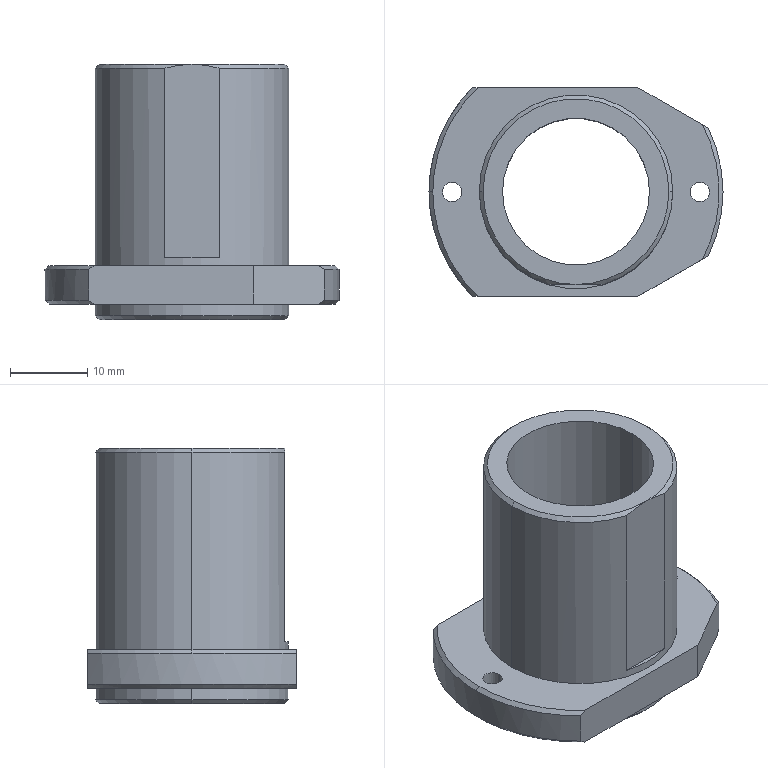Part | SolidWorks | features ICE 5, Chamfer 1, Cut 1, Extrusion 1, HoleWzd 1, MirrorPattern 1 | 1 solid | 34 faces | box 38 x 27 x 33 mm | volume 8754 mm3 | cylinder 13 | cone 11 | plane 10 | commonest cylinder face diameters 2.5 x4 25 x4 38 x3 19 x2
STEP:
#1=CARTESIAN_POINT('',(17.25,0.,-5.));
#2=VERTEX_POINT('',#1);
#3=CARTESIAN_POINT('',(14.75,0.,-5.));
#4=VERTEX_POINT('',#3);
#5=CARTESIAN_POINT('',(16.,0.,-5.));
#6=DIRECTION('',(0.,0.,-1.));
#7=DIRECTION('',(-1.,0.,0.));
#8=AXIS2_PLACEMENT_3D('',#5,#6,#7);
#9=CIRCLE('',#8,1.25);
#10=EDGE_CURVE('',#2,#4,#9,.T.);
#11=ORIENTED_EDGE('',*,*,#10,.T.);
#12=CARTESIAN_POINT('',(14.75,0.,0.));
#13=VERTEX_POINT('',#12);
#14=CARTESIAN_POINT('',(14.75,0.,0.));
#15=DIRECTION('',(0.,0.,1.));
#16=VECTOR('',#15,1000.);
#17=LINE('',#14,#16);
#18=EDGE_CURVE('',#4,#13,#17,.T.);
#19=ORIENTED_EDGE('',*,*,#18,.T.);
#20=CARTESIAN_POINT('',(17.25,0.,0.));
#21=VERTEX_POINT('',#20);
#22=CARTESIAN_POINT('',(16.,0.,0.));
#23=DIRECTION('',(0.,0.,1.));
#24=DIRECTION('',(1.,0.,0.));
#25=AXIS2_PLACEMENT_3D('',#22,#23,#24);
#26=CIRCLE('',#25,1.25);
#27=EDGE_CURVE('',#13,#21,#26,.T.);
#28=ORIENTED_EDGE('',*,*,#27,.T.);
#29=CARTESIAN_POINT('',(17.25,0.,0.));
#30=DIRECTION('',(0.,0.,1.));
#31=VECTOR('',#30,1000.);
#32=LINE('',#29,#31);
#33=EDGE_CURVE('',#2,#21,#32,.T.);
#34=ORIENTED_EDGE('',*,*,#33,.F.);
#35=EDGE_LOOP('',(#11,#19,#28,#34));
#36=FACE_OUTER_BOUND('',#35,.T.);
#37=CARTESIAN_POINT('',(16.,0.,0.));
#38=DIRECTION('',(0.,0.,1.));
#39=DIRECTION('',(1.,0.,0.));
#40=AXIS2_PLACEMENT_3D('',#37,#38,#39);
#41=CYLINDRICAL_SURFACE('',#40,1.25);
#42=ADVANCED_FACE('',(#36),#41,.F.);
#43=CARTESIAN_POINT('',(-14.75,0.,-5.));
#44=VERTEX_POINT('',#43);
#45=CARTESIAN_POINT('',(-17.25,0.,-5.));
#46=VERTEX_POINT('',#45);
#47=CARTESIAN_POINT('',(-16.,0.,-5.));
#48=DIRECTION('',(0.,0.,-1.));
#49=DIRECTION('',(-1.,0.,0.));
#50=AXIS2_PLACEMENT_3D('',#47,#48,#49);
#51=CIRCLE('',#50,1.25);
#52=EDGE_CURVE('',#44,#46,#51,.T.);
#53=ORIENTED_EDGE('',*,*,#52,.T.);
#54=CARTESIAN_POINT('',(-17.25,0.,0.));
#55=VERTEX_POINT('',#54);
#56=CARTESIAN_POINT('',(-17.25,0.,0.));
#57=DIRECTION('',(0.,0.,1.));
#58=VECTOR('',#57,1000.);
#59=LINE('',#56,#58);
#60=EDGE_CURVE('',#46,#55,#59,.T.);
#61=ORIENTED_EDGE('',*,*,#60,.T.);
#62=CARTESIAN_POINT('',(-14.75,0.,0.));
#63=VERTEX_POINT('',#62);
#64=CARTESIAN_POINT('',(-16.,0.,0.));
#65=DIRECTION('',(0.,0.,1.));
#66=DIRECTION('',(1.,0.,0.));
#67=AXIS2_PLACEMENT_3D('',#64,#65,#66);
#68=CIRCLE('',#67,1.25);
#69=EDGE_CURVE('',#55,#63,#68,.T.);
#70=ORIENTED_EDGE('',*,*,#69,.T.);
#71=CARTESIAN_POINT('',(-14.75,0.,0.));
#72=DIRECTION('',(0.,0.,1.));
#73=VECTOR('',#72,1000.);
#74=LINE('',#71,#73);
#75=EDGE_CURVE('',#44,#63,#74,.T.);
#76=ORIENTED_EDGE('',*,*,#75,.F.);
#77=EDGE_LOOP('',(#53,#61,#70,#76));
#78=FACE_OUTER_BOUND('',#77,.T.);
#79=CARTESIAN_POINT('',(-16.,0.,0.));
#80=DIRECTION('',(0.,0.,1.));
#81=DIRECTION('',(1.,0.,0.));
#82=AXIS2_PLACEMENT_3D('',#79,#80,#81);
#83=CYLINDRICAL_SURFACE('',#82,1.25);
#84=ADVANCED_FACE('',(#78),#83,.F.);
#85=CARTESIAN_POINT('',(-9.5,0.,-7.));
#86=VERTEX_POINT('',#85);
#87=CARTESIAN_POINT('',(9.5,0.,-7.));
#88=VERTEX_POINT('',#87);
#89=CARTESIAN_POINT('',(0.,0.,-7.));
#90=DIRECTION('',(0.,0.,1.));
#91=DIRECTION('',(1.,0.,0.));
#92=AXIS2_PLACEMENT_3D('',#89,#90,#91);
#93=CIRCLE('',#92,9.5);
#94=EDGE_CURVE('',#86,#88,#93,.T.);
#95=ORIENTED_EDGE('',*,*,#94,.F.);
#96=CARTESIAN_POINT('',(-9.5,0.,26.));
#97=VERTEX_POINT('',#96);
#98=CARTESIAN_POINT('',(-9.5,0.,-7.));
#99=DIRECTION('',(0.,0.,1.));
#100=VECTOR('',#99,1000.);
#101=LINE('',#98,#100);
#102=EDGE_CURVE('',#86,#97,#101,.T.);
#103=ORIENTED_EDGE('',*,*,#102,.T.);
#104=CARTESIAN_POINT('',(9.5,0.,26.));
#105=VERTEX_POINT('',#104);
#106=CARTESIAN_POINT('',(0.,0.,26.));
#107=DIRECTION('',(0.,0.,1.));
#108=DIRECTION('',(1.,0.,0.));
#109=AXIS2_PLACEMENT_3D('',#106,#107,#108);
#110=CIRCLE('',#109,9.5);
#111=EDGE_CURVE('',#97,#105,#110,.T.);
#112=ORIENTED_EDGE('',*,*,#111,.T.);
#113=CARTESIAN_POINT('',(9.5,0.,-7.));
#114=DIRECTION('',(0.,0.,1.));
#115=VECTOR('',#114,1000.);
#116=LINE('',#113,#115);
#117=EDGE_CURVE('',#88,#105,#116,.T.);
#118=ORIENTED_EDGE('',*,*,#117,.F.);
#119=EDGE_LOOP('',(#95,#103,#112,#118));
#120=FACE_OUTER_BOUND('',#119,.T.);
#121=CARTESIAN_POINT('',(0.,0.,-7.));
#122=DIRECTION('',(0.,0.,1.));
#123=DIRECTION('',(1.,0.,0.));
#124=AXIS2_PLACEMENT_3D('',#121,#122,#123);
#125=CYLINDRICAL_SURFACE('',#124,9.5);
#126=ADVANCED_FACE('',(#120),#125,.F.);
#127=CARTESIAN_POINT('',(-12.,0.,-7.));
#128=VERTEX_POINT('',#127);
#129=CARTESIAN_POINT('',(12.,0.,-7.));
#130=VERTEX_POINT('',#129);
#131=CARTESIAN_POINT('',(0.,0.,-7.));
#132=DIRECTION('',(0.,0.,-1.));
#133=DIRECTION('',(-1.,0.,0.));
#134=AXIS2_PLACEMENT_3D('',#131,#132,#133);
#135=CIRCLE('',#134,12.);
#136=EDGE_CURVE('',#128,#130,#135,.T.);
#137=ORIENTED_EDGE('',*,*,#136,.F.);
#138=CARTESIAN_POINT('',(-12.5,0.,-6.5));
#139=VERTEX_POINT('',#138);
#140=CARTESIAN_POINT('',(-12.,0.,-7.));
#141=DIRECTION('',(-0.7071,0.,0.7071));
#142=VECTOR('',#141,1000.);
#143=LINE('',#140,#142);
#144=EDGE_CURVE('',#128,#139,#143,.T.);
#145=ORIENTED_EDGE('',*,*,#144,.T.);
#146=CARTESIAN_POINT('',(12.5,0.,-6.5));
#147=VERTEX_POINT('',#146);
#148=CARTESIAN_POINT('',(0.,0.,-6.5));
#149=DIRECTION('',(0.,0.,1.));
#150=DIRECTION('',(-1.,0.,0.));
#151=AXIS2_PLACEMENT_3D('',#148,#149,#150);
#152=CIRCLE('',#151,12.5);
#153=EDGE_CURVE('',#147,#139,#152,.T.);
#154=ORIENTED_EDGE('',*,*,#153,.F.);
#155=CARTESIAN_POINT('',(12.,0.,-7.));
#156=DIRECTION('',(0.7071,0.,0.7071));
#157=VECTOR('',#156,1000.);
#158=LINE('',#155,#157);
#159=EDGE_CURVE('',#130,#147,#158,.T.);
#160=ORIENTED_EDGE('',*,*,#159,.F.);
#161=EDGE_LOOP('',(#137,#145,#154,#160));
#162=FACE_OUTER_BOUND('',#161,.T.);
#163=CARTESIAN_POINT('',(0.,0.,-7.));
#164=DIRECTION('',(0.,0.,1.));
#165=DIRECTION('',(1.,0.,0.));
#166=AXIS2_PLACEMENT_3D('',#163,#164,#165);
#167=CONICAL_SURFACE('',#166,12.,0.7854);
#168=ADVANCED_FACE('',(#162),#167,.T.);
#169=CARTESIAN_POINT('',(12.,0.,26.));
#170=VERTEX_POINT('',#169);
#171=CARTESIAN_POINT('',(-12.,0.,26.));
#172=VERTEX_POINT('',#171);
#173=CARTESIAN_POINT('',(0.,0.,26.));
#174=DIRECTION('',(0.,0.,1.));
#175=DIRECTION('',(1.,0.,0.));
#176=AXIS2_PLACEMENT_3D('',#173,#174,#175);
#177=CIRCLE('',#176,12.);
#178=EDGE_CURVE('',#170,#172,#177,.T.);
#179=ORIENTED_EDGE('',*,*,#178,.F.);
#180=CARTESIAN_POINT('',(12.5,0.,25.5));
#181=VERTEX_POINT('',#180);
#182=CARTESIAN_POINT('',(12.,0.,26.));
#183=DIRECTION('',(0.7071,0.,-0.7071));
#184=VECTOR('',#183,1000.);
#185=LINE('',#182,#184);
#186=EDGE_CURVE('',#170,#181,#185,.T.);
#187=ORIENTED_EDGE('',*,*,#186,.T.);
#188=CARTESIAN_POINT('',(-12.5,0.,25.5));
#189=VERTEX_POINT('',#188);
#190=CARTESIAN_POINT('',(0.,0.,25.5));
#191=DIRECTION('',(0.,0.,-1.));
#192=DIRECTION('',(1.,0.,0.));
#193=AXIS2_PLACEMENT_3D('',#190,#191,#192);
#194=CIRCLE('',#193,12.5);
#195=EDGE_CURVE('',#189,#181,#194,.T.);
#196=ORIENTED_EDGE('',*,*,#195,.F.);
#197=CARTESIAN_POINT('',(-12.,0.,26.));
#198=DIRECTION('',(-0.7071,0.,-0.7071));
#199=VECTOR('',#198,1000.);
#200=LINE('',#197,#199);
#201=EDGE_CURVE('',#172,#189,#200,.T.);
#202=ORIENTED_EDGE('',*,*,#201,.F.);
#203=EDGE_LOOP('',(#179,#187,#196,#202));
#204=FACE_OUTER_BOUND('',#203,.T.);
#205=CARTESIAN_POINT('',(0.,0.,26.));
#206=DIRECTION('',(0.,0.,-1.));
#207=DIRECTION('',(-1.,0.,0.));
#208=AXIS2_PLACEMENT_3D('',#205,#206,#207);
#209=CONICAL_SURFACE('',#208,12.,0.7854);
#210=ADVANCED_FACE('',(#204),#209,.T.);
#211=CARTESIAN_POINT('',(0.,-12.,26.));
#212=VERTEX_POINT('',#211);
#213=CARTESIAN_POINT('',(0.,0.,26.));
#214=DIRECTION('',(0.,0.,1.));
#215=DIRECTION('',(1.,0.,0.));
#216=AXIS2_PLACEMENT_3D('',#213,#214,#215);
#217=CIRCLE('',#216,12.);
#218=EDGE_CURVE('',#172,#212,#217,.T.);
#219=ORIENTED_EDGE('',*,*,#218,.F.);
#220=ORIENTED_EDGE('',*,*,#201,.T.);
#221=CARTESIAN_POINT('',(-3.5,-12.,25.5));
#222=VERTEX_POINT('',#221);
#223=CARTESIAN_POINT('',(0.,0.,25.5));
#224=DIRECTION('',(0.,0.,-1.));
#225=DIRECTION('',(1.,0.,0.));
#226=AXIS2_PLACEMENT_3D('',#223,#224,#225);
#227=CIRCLE('',#226,12.5);
#228=EDGE_CURVE('',#222,#189,#227,.T.);
#229=ORIENTED_EDGE('',*,*,#228,.F.);
#230=CARTESIAN_POINT('',(0.,-12.,26.));
#231=CARTESIAN_POINT('',(-0.5923,-12.,26.));
#232=CARTESIAN_POINT('',(-1.18,-12.,25.956));
#233=CARTESIAN_POINT('',(-2.055,-12.,25.829));
#234=CARTESIAN_POINT('',(-2.346,-12.,25.776));
#235=CARTESIAN_POINT('',(-2.925,-12.,25.652));
#236=CARTESIAN_POINT('',(-3.215,-12.,25.58));
#237=CARTESIAN_POINT('',(-3.5,-12.,25.5));
#238=B_SPLINE_CURVE_WITH_KNOTS('',3,(#230,#231,#232,#233,#234,#235,#236,#237),.UNSPECIFIED.,.F.,.F.,(4,2,2,4),(0.01538,0.01713,0.018,0.01888),.UNSPECIFIED.);
#239=EDGE_CURVE('',#212,#222,#238,.T.);
#240=ORIENTED_EDGE('',*,*,#239,.F.);
#241=EDGE_LOOP('',(#219,#220,#229,#240));
#242=FACE_OUTER_BOUND('',#241,.T.);
#243=CARTESIAN_POINT('',(0.,0.,26.));
#244=DIRECTION('',(0.,0.,-1.));
#245=DIRECTION('',(-1.,0.,0.));
#246=AXIS2_PLACEMENT_3D('',#243,#244,#245);
#247=CONICAL_SURFACE('',#246,12.,0.7854);
#248=ADVANCED_FACE('',(#242),#247,.T.);
#249=ORIENTED_EDGE('',*,*,#153,.T.);
#250=CARTESIAN_POINT('',(-12.5,0.,-5.));
#251=VERTEX_POINT('',#250);
#252=CARTESIAN_POINT('',(-12.5,0.,-7.));
#253=DIRECTION('',(0.,0.,1.));
#254=VECTOR('',#253,1000.);
#255=LINE('',#252,#254);
#256=EDGE_CURVE('',#139,#251,#255,.T.);
#257=ORIENTED_EDGE('',*,*,#256,.T.);
#258=CARTESIAN_POINT('',(12.5,0.,-5.));
#259=VERTEX_POINT('',#258);
#260=CARTESIAN_POINT('',(0.,0.,-5.));
#261=DIRECTION('',(0.,0.,-1.));
#262=DIRECTION('',(-1.,0.,0.));
#263=AXIS2_PLACEMENT_3D('',#260,#261,#262);
#264=CIRCLE('',#263,12.5);
#265=EDGE_CURVE('',#251,#259,#264,.T.);
#266=ORIENTED_EDGE('',*,*,#265,.T.);
#267=CARTESIAN_POINT('',(12.5,0.,-7.));
#268=DIRECTION('',(0.,0.,1.));
#269=VECTOR('',#268,1000.);
#270=LINE('',#267,#269);
#271=EDGE_CURVE('',#147,#259,#270,.T.);
#272=ORIENTED_EDGE('',*,*,#271,.F.);
#273=EDGE_LOOP('',(#249,#257,#266,#272));
#274=FACE_OUTER_BOUND('',#273,.T.);
#275=CARTESIAN_POINT('',(0.,0.,-7.));
#276=DIRECTION('',(0.,0.,1.));
#277=DIRECTION('',(1.,0.,0.));
#278=AXIS2_PLACEMENT_3D('',#275,#276,#277);
#279=CYLINDRICAL_SURFACE('',#278,12.5);
#280=ADVANCED_FACE('',(#274),#279,.T.);
#281=ORIENTED_EDGE('',*,*,#195,.T.);
#282=CARTESIAN_POINT('',(12.5,0.,0.));
#283=VERTEX_POINT('',#282);
#284=CARTESIAN_POINT('',(12.5,0.,26.));
#285=DIRECTION('',(0.,0.,-1.));
#286=VECTOR('',#285,1000.);
#287=LINE('',#284,#286);
#288=EDGE_CURVE('',#181,#283,#287,.T.);
#289=ORIENTED_EDGE('',*,*,#288,.T.);
#290=CARTESIAN_POINT('',(-12.5,0.,0.));
#291=VERTEX_POINT('',#290);
#292=CARTESIAN_POINT('',(0.,0.,0.));
#293=DIRECTION('',(0.,0.,-1.));
#294=DIRECTION('',(-1.,0.,0.));
#295=AXIS2_PLACEMENT_3D('',#292,#293,#294);
#296=CIRCLE('',#295,12.5);
#297=EDGE_CURVE('',#291,#283,#296,.T.);
#298=ORIENTED_EDGE('',*,*,#297,.F.);
#299=CARTESIAN_POINT('',(-12.5,0.,26.));
#300=DIRECTION('',(0.,0.,-1.));
#301=VECTOR('',#300,1000.);
#302=LINE('',#299,#301);
#303=EDGE_CURVE('',#189,#291,#302,.T.);
#304=ORIENTED_EDGE('',*,*,#303,.F.);
#305=EDGE_LOOP('',(#281,#289,#298,#304));
#306=FACE_OUTER_BOUND('',#305,.T.);
#307=CARTESIAN_POINT('',(0.,0.,26.));
#308=DIRECTION('',(0.,0.,-1.));
#309=DIRECTION('',(-1.,0.,0.));
#310=AXIS2_PLACEMENT_3D('',#307,#308,#309);
#311=CYLINDRICAL_SURFACE('',#310,12.5);
#312=ADVANCED_FACE('',(#306),#311,.T.);
#313=CARTESIAN_POINT('',(-18.5,0.,0.));
#314=VERTEX_POINT('',#313);
#315=CARTESIAN_POINT('',(-12.649,-13.5,0.));
#316=VERTEX_POINT('',#315);
#317=CARTESIAN_POINT('',(0.,0.,0.));
#318=DIRECTION('',(0.,0.,1.));
#319=DIRECTION('',(-1.,0.,0.));
#320=AXIS2_PLACEMENT_3D('',#317,#318,#319);
#321=CIRCLE('',#320,18.5);
#322=EDGE_CURVE('',#314,#316,#321,.T.);
#323=ORIENTED_EDGE('',*,*,#322,.F.);
#324=CARTESIAN_POINT('',(-19.,0.,-0.5));
#325=VERTEX_POINT('',#324);
#326=CARTESIAN_POINT('',(-19.,0.,-0.5));
#327=DIRECTION('',(-0.7071,0.,-0.7071));
#328=VECTOR('',#327,1000.);
#329=LINE('',#326,#328);
#330=EDGE_CURVE('',#314,#325,#329,.T.);
#331=ORIENTED_EDGE('',*,*,#330,.T.);
#332=CARTESIAN_POINT('',(-13.37,-13.5,-0.5));
#333=VERTEX_POINT('',#332);
#334=CARTESIAN_POINT('',(0.,0.,-0.5));
#335=DIRECTION('',(0.,0.,-1.));
#336=DIRECTION('',(-1.,0.,0.));
#337=AXIS2_PLACEMENT_3D('',#334,#335,#336);
#338=CIRCLE('',#337,19.);
#339=EDGE_CURVE('',#333,#325,#338,.T.);
#340=ORIENTED_EDGE('',*,*,#339,.F.);
#341=CARTESIAN_POINT('',(-12.649,-13.5,0.));
#342=CARTESIAN_POINT('',(-12.891,-13.5,-0.1651));
#343=CARTESIAN_POINT('',(-13.131,-13.5,-0.3319));
#344=CARTESIAN_POINT('',(-13.37,-13.5,-0.5));
#345=B_SPLINE_CURVE_WITH_KNOTS('',3,(#341,#342,#343,#344),.UNSPECIFIED.,.F.,.F.,(4,4),(0.06294,0.0638),.UNSPECIFIED.);
#346=EDGE_CURVE('',#316,#333,#345,.T.);
#347=ORIENTED_EDGE('',*,*,#346,.F.);
#348=EDGE_LOOP('',(#323,#331,#340,#347));
#349=FACE_OUTER_BOUND('',#348,.T.);
#350=CARTESIAN_POINT('',(0.,0.,-0.5));
#351=DIRECTION('',(0.,0.,-1.));
#352=DIRECTION('',(-1.,0.,0.));
#353=AXIS2_PLACEMENT_3D('',#350,#351,#352);
#354=CONICAL_SURFACE('',#353,19.,0.7854);
#355=ADVANCED_FACE('',(#349),#354,.T.);
#356=CARTESIAN_POINT('',(18.5,0.,-5.));
#357=VERTEX_POINT('',#356);
#358=CARTESIAN_POINT('',(16.332,-8.689,-5.));
#359=VERTEX_POINT('',#358);
#360=CARTESIAN_POINT('',(0.,0.,-5.));
#361=DIRECTION('',(0.,0.,-1.));
#362=DIRECTION('',(-1.,0.,0.));
#363=AXIS2_PLACEMENT_3D('',#360,#361,#362);
#364=CIRCLE('',#363,18.5);
#365=EDGE_CURVE('',#357,#359,#364,.T.);
#366=ORIENTED_EDGE('',*,*,#365,.F.);
#367=CARTESIAN_POINT('',(19.,0.,-4.5));
#368=VERTEX_POINT('',#367);
#369=CARTESIAN_POINT('',(18.5,0.,-5.));
#370=DIRECTION('',(0.7071,0.,0.7071));
#371=VECTOR('',#370,1000.);
#372=LINE('',#369,#371);
#373=EDGE_CURVE('',#357,#368,#372,.T.);
#374=ORIENTED_EDGE('',*,*,#373,.T.);
#375=CARTESIAN_POINT('',(17.124,-8.232,-4.5));
#376=VERTEX_POINT('',#375);
#377=CARTESIAN_POINT('',(0.,0.,-4.5));
#378=DIRECTION('',(0.,0.,1.));
#379=DIRECTION('',(-1.,0.,0.));
#380=AXIS2_PLACEMENT_3D('',#377,#378,#379);
#381=CIRCLE('',#380,19.);
#382=EDGE_CURVE('',#376,#368,#381,.T.);
#383=ORIENTED_EDGE('',*,*,#382,.F.);
#384=CARTESIAN_POINT('',(17.124,-8.232,-4.5));
#385=CARTESIAN_POINT('',(16.862,-8.383,-4.67));
#386=CARTESIAN_POINT('',(16.598,-8.536,-4.837));
#387=CARTESIAN_POINT('',(16.332,-8.689,-5.));
#388=B_SPLINE_CURVE_WITH_KNOTS('',3,(#384,#385,#386,#387),.UNSPECIFIED.,.F.,.F.,(4,4),(0.0104,0.01144),.UNSPECIFIED.);
#389=EDGE_CURVE('',#376,#359,#388,.T.);
#390=ORIENTED_EDGE('',*,*,#389,.T.);
#391=EDGE_LOOP('',(#366,#374,#383,#390));
#392=FACE_OUTER_BOUND('',#391,.T.);
#393=CARTESIAN_POINT('',(0.,0.,-5.));
#394=DIRECTION('',(0.,0.,1.));
#395=DIRECTION('',(1.,0.,0.));
#396=AXIS2_PLACEMENT_3D('',#393,#394,#395);
#397=CONICAL_SURFACE('',#396,18.5,0.7854);
#398=ADVANCED_FACE('',(#392),#397,.T.);
#399=ORIENTED_EDGE('',*,*,#382,.T.);
#400=CARTESIAN_POINT('',(19.,0.,-0.5));
#401=VERTEX_POINT('',#400);
#402=CARTESIAN_POINT('',(19.,0.,-5.));
#403=DIRECTION('',(0.,0.,1.));
#404=VECTOR('',#403,1000.);
#405=LINE('',#402,#404);
#406=EDGE_CURVE('',#368,#401,#405,.T.);
#407=ORIENTED_EDGE('',*,*,#406,.T.);
#408=CARTESIAN_POINT('',(17.124,-8.232,-0.5));
#409=VERTEX_POINT('',#408);
#410=CARTESIAN_POINT('',(0.,0.,-0.5));
#411=DIRECTION('',(0.,0.,-1.));
#412=DIRECTION('',(-1.,0.,0.));
#413=AXIS2_PLACEMENT_3D('',#410,#411,#412);
#414=CIRCLE('',#413,19.);
#415=EDGE_CURVE('',#401,#409,#414,.T.);
#416=ORIENTED_EDGE('',*,*,#415,.T.);
#417=CARTESIAN_POINT('',(17.124,-8.232,-5.));
#418=DIRECTION('',(0.,0.,1.));
#419=VECTOR('',#418,1000.);
#420=LINE('',#417,#419);
#421=EDGE_CURVE('',#376,#409,#420,.T.);
#422=ORIENTED_EDGE('',*,*,#421,.F.);
#423=EDGE_LOOP('',(#399,#407,#416,#422));
#424=FACE_OUTER_BOUND('',#423,.T.);
#425=CARTESIAN_POINT('',(0.,0.,-5.));
#426=DIRECTION('',(0.,0.,1.));
#427=DIRECTION('',(1.,0.,0.));
#428=AXIS2_PLACEMENT_3D('',#425,#426,#427);
#429=CYLINDRICAL_SURFACE('',#428,19.);
#430=ADVANCED_FACE('',(#424),#429,.T.);
#431=ORIENTED_EDGE('',*,*,#406,.F.);
#432=CARTESIAN_POINT('',(17.124,8.232,-4.5));
#433=VERTEX_POINT('',#432);
#434=CARTESIAN_POINT('',(0.,0.,-4.5));
#435=DIRECTION('',(0.,0.,1.));
#436=DIRECTION('',(-1.,0.,0.));
#437=AXIS2_PLACEMENT_3D('',#434,#435,#436);
#438=CIRCLE('',#437,19.);
#439=EDGE_CURVE('',#368,#433,#438,.T.);
#440=ORIENTED_EDGE('',*,*,#439,.T.);
#441=CARTESIAN_POINT('',(17.124,8.232,-0.5));
#442=VERTEX_POINT('',#441);
#443=CARTESIAN_POINT('',(17.124,8.232,-5.));
#444=DIRECTION('',(0.,0.,1.));
#445=VECTOR('',#444,1000.);
#446=LINE('',#443,#445);
#447=EDGE_CURVE('',#433,#442,#446,.T.);
#448=ORIENTED_EDGE('',*,*,#447,.T.);
#449=CARTESIAN_POINT('',(0.,0.,-0.5));
#450=DIRECTION('',(0.,0.,-1.));
#451=DIRECTION('',(-1.,0.,0.));
#452=AXIS2_PLACEMENT_3D('',#449,#450,#451);
#453=CIRCLE('',#452,19.);
#454=EDGE_CURVE('',#442,#401,#453,.T.);
#455=ORIENTED_EDGE('',*,*,#454,.T.);
#456=EDGE_LOOP('',(#431,#440,#448,#455));
#457=FACE_OUTER_BOUND('',#456,.T.);
#458=CARTESIAN_POINT('',(0.,0.,-5.));
#459=DIRECTION('',(0.,0.,1.));
#460=DIRECTION('',(1.,0.,0.));
#461=AXIS2_PLACEMENT_3D('',#458,#459,#460);
#462=CYLINDRICAL_SURFACE('',#461,19.);
#463=ADVANCED_FACE('',(#457),#462,.T.);
#464=ORIENTED_EDGE('',*,*,#373,.F.);
#465=CARTESIAN_POINT('',(16.332,8.689,-5.));
#466=VERTEX_POINT('',#465);
#467=CARTESIAN_POINT('',(0.,0.,-5.));
#468=DIRECTION('',(0.,0.,-1.));
#469=DIRECTION('',(-1.,0.,0.));
#470=AXIS2_PLACEMENT_3D('',#467,#468,#469);
#471=CIRCLE('',#470,18.5);
#472=EDGE_CURVE('',#466,#357,#471,.T.);
#473=ORIENTED_EDGE('',*,*,#472,.F.);
#474=CARTESIAN_POINT('',(17.124,8.232,-4.5));
#475=CARTESIAN_POINT('',(16.862,8.383,-4.67));
#476=CARTESIAN_POINT('',(16.598,8.536,-4.837));
#477=CARTESIAN_POINT('',(16.332,8.689,-5.));
#478=B_SPLINE_CURVE_WITH_KNOTS('',3,(#474,#475,#476,#477),.UNSPECIFIED.,.F.,.F.,(4,4),(0.0104,0.01144),.UNSPECIFIED.);
#479=EDGE_CURVE('',#433,#466,#478,.T.);
#480=ORIENTED_EDGE('',*,*,#479,.F.);
#481=ORIENTED_EDGE('',*,*,#439,.F.);
#482=EDGE_LOOP('',(#464,#473,#480,#481));
#483=FACE_OUTER_BOUND('',#482,.T.);
#484=CARTESIAN_POINT('',(0.,0.,-5.));
#485=DIRECTION('',(0.,0.,1.));
#486=DIRECTION('',(1.,0.,0.));
#487=AXIS2_PLACEMENT_3D('',#484,#485,#486);
#488=CONICAL_SURFACE('',#487,18.5,0.7854);
#489=ADVANCED_FACE('',(#483),#488,.T.);
#490=CARTESIAN_POINT('',(0.,0.,-5.));
#491=DIRECTION('',(0.,0.,-1.));
#492=DIRECTION('',(-1.,0.,0.));
#493=AXIS2_PLACEMENT_3D('',#490,#491,#492);
#494=CIRCLE('',#493,12.5);
#495=EDGE_CURVE('',#259,#251,#494,.T.);
#496=ORIENTED_EDGE('',*,*,#495,.F.);
#497=ORIENTED_EDGE('',*,*,#265,.F.);
#498=EDGE_LOOP('',(#496,#497));
#499=FACE_BOUND('',#498,.T.);
#500=ORIENTED_EDGE('',*,*,#52,.F.);
#501=CARTESIAN_POINT('',(-16.,0.,-5.));
#502=DIRECTION('',(0.,0.,-1.));
#503=DIRECTION('',(-1.,0.,0.));
#504=AXIS2_PLACEMENT_3D('',#501,#502,#503);
#505=CIRCLE('',#504,1.25);
#506=EDGE_CURVE('',#46,#44,#505,.T.);
#507=ORIENTED_EDGE('',*,*,#506,.F.);
#508=EDGE_LOOP('',(#500,#507));
#509=FACE_BOUND('',#508,.T.);
#510=ORIENTED_EDGE('',*,*,#10,.F.);
#511=CARTESIAN_POINT('',(16.,0.,-5.));
#512=DIRECTION('',(0.,0.,-1.));
#513=DIRECTION('',(-1.,0.,0.));
#514=AXIS2_PLACEMENT_3D('',#511,#512,#513);
#515=CIRCLE('',#514,1.25);
#516=EDGE_CURVE('',#4,#2,#515,.T.);
#517=ORIENTED_EDGE('',*,*,#516,.F.);
#518=EDGE_LOOP('',(#510,#517));
#519=FACE_BOUND('',#518,.T.);
#520=ORIENTED_EDGE('',*,*,#472,.T.);
#521=ORIENTED_EDGE('',*,*,#365,.T.);
#522=CARTESIAN_POINT('',(8.,-13.5,-5.));
#523=VERTEX_POINT('',#522);
#524=CARTESIAN_POINT('',(7.846,-13.589,-5.));
#525=DIRECTION('',(-0.866,-0.5,0.));
#526=VECTOR('',#525,1000.);
#527=LINE('',#524,#526);
#528=EDGE_CURVE('',#359,#523,#527,.T.);
#529=ORIENTED_EDGE('',*,*,#528,.T.);
#530=CARTESIAN_POINT('',(-12.649,-13.5,-5.));
#531=VERTEX_POINT('',#530);
#532=CARTESIAN_POINT('',(0.,-13.5,-5.));
#533=DIRECTION('',(1.,0.,0.));
#534=VECTOR('',#533,1000.);
#535=LINE('',#532,#534);
#536=EDGE_CURVE('',#531,#523,#535,.T.);
#537=ORIENTED_EDGE('',*,*,#536,.F.);
#538=CARTESIAN_POINT('',(-12.649,13.5,-5.));
#539=VERTEX_POINT('',#538);
#540=CARTESIAN_POINT('',(0.,0.,-5.));
#541=DIRECTION('',(0.,0.,-1.));
#542=DIRECTION('',(-1.,0.,0.));
#543=AXIS2_PLACEMENT_3D('',#540,#541,#542);
#544=CIRCLE('',#543,18.5);
#545=EDGE_CURVE('',#531,#539,#544,.T.);
#546=ORIENTED_EDGE('',*,*,#545,.T.);
#547=CARTESIAN_POINT('',(8.,13.5,-5.));
#548=VERTEX_POINT('',#547);
#549=CARTESIAN_POINT('',(0.,13.5,-5.));
#550=DIRECTION('',(-1.,0.,0.));
#551=VECTOR('',#550,1000.);
#552=LINE('',#549,#551);
#553=EDGE_CURVE('',#548,#539,#552,.T.);
#554=ORIENTED_EDGE('',*,*,#553,.F.);
#555=CARTESIAN_POINT('',(7.846,13.589,-5.));
#556=DIRECTION('',(-0.866,0.5,0.));
#557=VECTOR('',#556,1000.);
#558=LINE('',#555,#557);
#559=EDGE_CURVE('',#466,#548,#558,.T.);
#560=ORIENTED_EDGE('',*,*,#559,.F.);
#561=EDGE_LOOP('',(#520,#521,#529,#537,#546,#554,#560));
#562=FACE_OUTER_BOUND('',#561,.T.);
#563=CARTESIAN_POINT('',(0.,0.,-5.));
#564=DIRECTION('',(0.,0.,-1.));
#565=DIRECTION('',(-1.,0.,0.));
#566=AXIS2_PLACEMENT_3D('',#563,#564,#565);
#567=PLANE('',#566);
#568=ADVANCED_FACE('',(#499,#509,#519,#562),#567,.T.);
#569=ORIENTED_EDGE('',*,*,#297,.T.);
#570=CARTESIAN_POINT('',(0.,0.,0.));
#571=DIRECTION('',(0.,0.,-1.));
#572=DIRECTION('',(-1.,0.,0.));
#573=AXIS2_PLACEMENT_3D('',#570,#571,#572);
#574=CIRCLE('',#573,12.5);
#575=EDGE_CURVE('',#283,#291,#574,.T.);
#576=ORIENTED_EDGE('',*,*,#575,.T.);
#577=EDGE_LOOP('',(#569,#576));
#578=FACE_BOUND('',#577,.T.);
#579=CARTESIAN_POINT('',(-16.,0.,0.));
#580=DIRECTION('',(0.,0.,1.));
#581=DIRECTION('',(1.,0.,0.));
#582=AXIS2_PLACEMENT_3D('',#579,#580,#581);
#583=CIRCLE('',#582,1.25);
#584=EDGE_CURVE('',#63,#55,#583,.T.);
#585=ORIENTED_EDGE('',*,*,#584,.F.);
#586=ORIENTED_EDGE('',*,*,#69,.F.);
#587=EDGE_LOOP('',(#585,#586));
#588=FACE_BOUND('',#587,.T.);
#589=CARTESIAN_POINT('',(16.,0.,0.));
#590=DIRECTION('',(0.,0.,1.));
#591=DIRECTION('',(1.,0.,0.));
#592=AXIS2_PLACEMENT_3D('',#589,#590,#591);
#593=CIRCLE('',#592,1.25);
#594=EDGE_CURVE('',#21,#13,#593,.T.);
#595=ORIENTED_EDGE('',*,*,#594,.F.);
#596=ORIENTED_EDGE('',*,*,#27,.F.);
#597=EDGE_LOOP('',(#595,#596));
#598=FACE_BOUND('',#597,.T.);
#599=CARTESIAN_POINT('',(8.,-13.5,0.));
#600=VERTEX_POINT('',#599);
#601=CARTESIAN_POINT('',(16.332,-8.689,0.));
#602=VERTEX_POINT('',#601);
#603=CARTESIAN_POINT('',(20.899,-6.053,0.));
#604=DIRECTION('',(0.866,0.5,0.));
#605=VECTOR('',#604,1000.);
#606=LINE('',#603,#605);
#607=EDGE_CURVE('',#600,#602,#606,.T.);
#608=ORIENTED_EDGE('',*,*,#607,.T.);
#609=CARTESIAN_POINT('',(16.332,8.689,0.));
#610=VERTEX_POINT('',#609);
#611=CARTESIAN_POINT('',(0.,0.,0.));
#612=DIRECTION('',(0.,0.,1.));
#613=DIRECTION('',(-1.,0.,0.));
#614=AXIS2_PLACEMENT_3D('',#611,#612,#613);
#615=CIRCLE('',#614,18.5);
#616=EDGE_CURVE('',#602,#610,#615,.T.);
#617=ORIENTED_EDGE('',*,*,#616,.T.);
#618=CARTESIAN_POINT('',(8.,13.5,0.));
#619=VERTEX_POINT('',#618);
#620=CARTESIAN_POINT('',(20.899,6.053,0.));
#621=DIRECTION('',(0.866,-0.5,0.));
#622=VECTOR('',#621,1000.);
#623=LINE('',#620,#622);
#624=EDGE_CURVE('',#619,#610,#623,.T.);
#625=ORIENTED_EDGE('',*,*,#624,.F.);
#626=CARTESIAN_POINT('',(-12.649,13.5,0.));
#627=VERTEX_POINT('',#626);
#628=CARTESIAN_POINT('',(27.33,13.5,0.));
#629=DIRECTION('',(1.,0.,0.));
#630=VECTOR('',#629,1000.);
#631=LINE('',#628,#630);
#632=EDGE_CURVE('',#627,#619,#631,.T.);
#633=ORIENTED_EDGE('',*,*,#632,.F.);
#634=CARTESIAN_POINT('',(0.,0.,0.));
#635=DIRECTION('',(0.,0.,1.));
#636=DIRECTION('',(-1.,0.,0.));
#637=AXIS2_PLACEMENT_3D('',#634,#635,#636);
#638=CIRCLE('',#637,18.5);
#639=EDGE_CURVE('',#627,#314,#638,.T.);
#640=ORIENTED_EDGE('',*,*,#639,.T.);
#641=ORIENTED_EDGE('',*,*,#322,.T.);
#642=CARTESIAN_POINT('',(27.95,-13.5,0.));
#643=DIRECTION('',(-1.,0.,0.));
#644=VECTOR('',#643,1000.);
#645=LINE('',#642,#644);
#646=EDGE_CURVE('',#600,#316,#645,.T.);
#647=ORIENTED_EDGE('',*,*,#646,.F.);
#648=EDGE_LOOP('',(#608,#617,#625,#633,#640,#641,#647));
#649=FACE_OUTER_BOUND('',#648,.T.);
#650=CARTESIAN_POINT('',(0.,0.,0.));
#651=DIRECTION('',(0.,0.,-1.));
#652=DIRECTION('',(-1.,0.,0.));
#653=AXIS2_PLACEMENT_3D('',#650,#651,#652);
#654=PLANE('',#653);
#655=ADVANCED_FACE('',(#578,#588,#598,#649),#654,.F.);
#656=ORIENTED_EDGE('',*,*,#616,.F.);
#657=CARTESIAN_POINT('',(16.332,-8.689,0.));
#658=CARTESIAN_POINT('',(16.598,-8.536,-0.1623));
#659=CARTESIAN_POINT('',(16.862,-8.384,-0.3293));
#660=CARTESIAN_POINT('',(17.124,-8.232,-0.5));
#661=B_SPLINE_CURVE_WITH_KNOTS('',3,(#657,#658,#659,#660),.UNSPECIFIED.,.F.,.F.,(4,4),(0.01154,0.01258),.UNSPECIFIED.);
#662=EDGE_CURVE('',#602,#409,#661,.T.);
#663=ORIENTED_EDGE('',*,*,#662,.T.);
#664=ORIENTED_EDGE('',*,*,#415,.F.);
#665=ORIENTED_EDGE('',*,*,#454,.F.);
#666=CARTESIAN_POINT('',(16.332,8.689,0.));
#667=CARTESIAN_POINT('',(16.598,8.536,-0.1623));
#668=CARTESIAN_POINT('',(16.862,8.384,-0.3293));
#669=CARTESIAN_POINT('',(17.124,8.232,-0.5));
#670=B_SPLINE_CURVE_WITH_KNOTS('',3,(#666,#667,#668,#669),.UNSPECIFIED.,.F.,.F.,(4,4),(0.01154,0.01258),.UNSPECIFIED.);
#671=EDGE_CURVE('',#610,#442,#670,.T.);
#672=ORIENTED_EDGE('',*,*,#671,.F.);
#673=EDGE_LOOP('',(#656,#663,#664,#665,#672));
#674=FACE_OUTER_BOUND('',#673,.T.);
#675=CARTESIAN_POINT('',(0.,0.,-0.5));
#676=DIRECTION('',(0.,0.,-1.));
#677=DIRECTION('',(-1.,0.,0.));
#678=AXIS2_PLACEMENT_3D('',#675,#676,#677);
#679=CONICAL_SURFACE('',#678,19.,0.7854);
#680=ADVANCED_FACE('',(#674),#679,.T.);
#681=CARTESIAN_POINT('',(8.,-13.5,-7.));
#682=DIRECTION('',(0.,0.,-1.));
#683=VECTOR('',#682,1000.);
#684=LINE('',#681,#683);
#685=EDGE_CURVE('',#600,#523,#684,.T.);
#686=ORIENTED_EDGE('',*,*,#685,.F.);
#687=ORIENTED_EDGE('',*,*,#646,.T.);
#688=ORIENTED_EDGE('',*,*,#346,.T.);
#689=CARTESIAN_POINT('',(-13.37,-13.5,-4.5));
#690=VERTEX_POINT('',#689);
#691=CARTESIAN_POINT('',(-13.37,-13.5,-5.));
#692=DIRECTION('',(0.,0.,1.));
#693=VECTOR('',#692,1000.);
#694=LINE('',#691,#693);
#695=EDGE_CURVE('',#690,#333,#694,.T.);
#696=ORIENTED_EDGE('',*,*,#695,.F.);
#697=CARTESIAN_POINT('',(-13.37,-13.5,-4.5));
#698=CARTESIAN_POINT('',(-13.131,-13.5,-4.668));
#699=CARTESIAN_POINT('',(-12.89,-13.5,-4.835));
#700=CARTESIAN_POINT('',(-12.649,-13.5,-5.));
#701=B_SPLINE_CURVE_WITH_KNOTS('',3,(#697,#698,#699,#700),.UNSPECIFIED.,.F.,.F.,(4,4),(0.03479,0.03567),.UNSPECIFIED.);
#702=EDGE_CURVE('',#690,#531,#701,.T.);
#703=ORIENTED_EDGE('',*,*,#702,.T.);
#704=ORIENTED_EDGE('',*,*,#536,.T.);
#705=EDGE_LOOP('',(#686,#687,#688,#696,#703,#704));
#706=FACE_OUTER_BOUND('',#705,.T.);
#707=CARTESIAN_POINT('',(27.95,-13.5,-7.));
#708=DIRECTION('',(0.,1.,0.));
#709=DIRECTION('',(-1.,0.,0.));
#710=AXIS2_PLACEMENT_3D('',#707,#708,#709);
#711=PLANE('',#710);
#712=ADVANCED_FACE('',(#706),#711,.F.);
#713=ORIENTED_EDGE('',*,*,#330,.F.);
#714=ORIENTED_EDGE('',*,*,#639,.F.);
#715=CARTESIAN_POINT('',(-13.37,13.5,-0.5));
#716=VERTEX_POINT('',#715);
#717=CARTESIAN_POINT('',(-13.37,13.5,-0.5));
#718=CARTESIAN_POINT('',(-13.131,13.5,-0.3317));
#719=CARTESIAN_POINT('',(-12.89,13.5,-0.165));
#720=CARTESIAN_POINT('',(-12.649,13.5,0.));
#721=B_SPLINE_CURVE_WITH_KNOTS('',3,(#717,#718,#719,#720),.UNSPECIFIED.,.F.,.F.,(4,4),(0.03479,0.03567),.UNSPECIFIED.);
#722=EDGE_CURVE('',#716,#627,#721,.T.);
#723=ORIENTED_EDGE('',*,*,#722,.F.);
#724=CARTESIAN_POINT('',(0.,0.,-0.5));
#725=DIRECTION('',(0.,0.,-1.));
#726=DIRECTION('',(-1.,0.,0.));
#727=AXIS2_PLACEMENT_3D('',#724,#725,#726);
#728=CIRCLE('',#727,19.);
#729=EDGE_CURVE('',#325,#716,#728,.T.);
#730=ORIENTED_EDGE('',*,*,#729,.F.);
#731=EDGE_LOOP('',(#713,#714,#723,#730));
#732=FACE_OUTER_BOUND('',#731,.T.);
#733=CARTESIAN_POINT('',(0.,0.,-0.5));
#734=DIRECTION('',(0.,0.,-1.));
#735=DIRECTION('',(-1.,0.,0.));
#736=AXIS2_PLACEMENT_3D('',#733,#734,#735);
#737=CONICAL_SURFACE('',#736,19.,0.7854);
#738=ADVANCED_FACE('',(#732),#737,.T.);
#739=ORIENTED_EDGE('',*,*,#288,.F.);
#740=CARTESIAN_POINT('',(3.5,-12.,25.5));
#741=VERTEX_POINT('',#740);
#742=CARTESIAN_POINT('',(0.,0.,25.5));
#743=DIRECTION('',(0.,0.,-1.));
#744=DIRECTION('',(1.,0.,0.));
#745=AXIS2_PLACEMENT_3D('',#742,#743,#744);
#746=CIRCLE('',#745,12.5);
#747=EDGE_CURVE('',#181,#741,#746,.T.);
#748=ORIENTED_EDGE('',*,*,#747,.T.);
#749=CARTESIAN_POINT('',(3.5,-12.,1.));
#750=VERTEX_POINT('',#749);
#751=CARTESIAN_POINT('',(3.5,-12.,26.));
#752=DIRECTION('',(0.,0.,-1.));
#753=VECTOR('',#752,1000.);
#754=LINE('',#751,#753);
#755=EDGE_CURVE('',#741,#750,#754,.T.);
#756=ORIENTED_EDGE('',*,*,#755,.T.);
#757=CARTESIAN_POINT('',(-3.5,-12.,1.));
#758=VERTEX_POINT('',#757);
#759=CARTESIAN_POINT('',(0.,0.,1.));
#760=DIRECTION('',(0.,0.,-1.));
#761=DIRECTION('',(-1.,0.,0.));
#762=AXIS2_PLACEMENT_3D('',#759,#760,#761);
#763=CIRCLE('',#762,12.5);
#764=EDGE_CURVE('',#750,#758,#763,.T.);
#765=ORIENTED_EDGE('',*,*,#764,.T.);
#766=CARTESIAN_POINT('',(-3.5,-12.,26.));
#767=DIRECTION('',(0.,0.,1.));
#768=VECTOR('',#767,1000.);
#769=LINE('',#766,#768);
#770=EDGE_CURVE('',#758,#222,#769,.T.);
#771=ORIENTED_EDGE('',*,*,#770,.T.);
#772=ORIENTED_EDGE('',*,*,#228,.T.);
#773=ORIENTED_EDGE('',*,*,#303,.T.);
#774=ORIENTED_EDGE('',*,*,#575,.F.);
#775=EDGE_LOOP('',(#739,#748,#756,#765,#771,#772,#773,#774));
#776=FACE_OUTER_BOUND('',#775,.T.);
#777=CARTESIAN_POINT('',(0.,0.,26.));
#778=DIRECTION('',(0.,0.,-1.));
#779=DIRECTION('',(-1.,0.,0.));
#780=AXIS2_PLACEMENT_3D('',#777,#778,#779);
#781=CYLINDRICAL_SURFACE('',#780,12.5);
#782=ADVANCED_FACE('',(#776),#781,.T.);
#783=CARTESIAN_POINT('',(0.,0.,26.));
#784=DIRECTION('',(0.,0.,1.));
#785=DIRECTION('',(1.,0.,0.));
#786=AXIS2_PLACEMENT_3D('',#783,#784,#785);
#787=CIRCLE('',#786,9.5);
#788=EDGE_CURVE('',#105,#97,#787,.T.);
#789=ORIENTED_EDGE('',*,*,#788,.F.);
#790=ORIENTED_EDGE('',*,*,#111,.F.);
#791=EDGE_LOOP('',(#789,#790));
#792=FACE_BOUND('',#791,.T.);
#793=CARTESIAN_POINT('',(0.,0.,26.));
#794=DIRECTION('',(0.,0.,1.));
#795=DIRECTION('',(1.,0.,0.));
#796=AXIS2_PLACEMENT_3D('',#793,#794,#795);
#797=CIRCLE('',#796,12.);
#798=EDGE_CURVE('',#212,#170,#797,.T.);
#799=ORIENTED_EDGE('',*,*,#798,.T.);
#800=ORIENTED_EDGE('',*,*,#178,.T.);
#801=ORIENTED_EDGE('',*,*,#218,.T.);
#802=EDGE_LOOP('',(#799,#800,#801));
#803=FACE_OUTER_BOUND('',#802,.T.);
#804=CARTESIAN_POINT('',(0.,0.,26.));
#805=DIRECTION('',(0.,0.,1.));
#806=DIRECTION('',(1.,0.,0.));
#807=AXIS2_PLACEMENT_3D('',#804,#805,#806);
#808=PLANE('',#807);
#809=ADVANCED_FACE('',(#792,#803),#808,.T.);
#810=ORIENTED_EDGE('',*,*,#339,.T.);
#811=ORIENTED_EDGE('',*,*,#729,.T.);
#812=CARTESIAN_POINT('',(-13.37,13.5,-4.5));
#813=VERTEX_POINT('',#812);
#814=CARTESIAN_POINT('',(-13.37,13.5,-5.));
#815=DIRECTION('',(0.,0.,-1.));
#816=VECTOR('',#815,1000.);
#817=LINE('',#814,#816);
#818=EDGE_CURVE('',#716,#813,#817,.T.);
#819=ORIENTED_EDGE('',*,*,#818,.T.);
#820=CARTESIAN_POINT('',(0.,0.,-4.5));
#821=DIRECTION('',(0.,0.,1.));
#822=DIRECTION('',(-1.,0.,0.));
#823=AXIS2_PLACEMENT_3D('',#820,#821,#822);
#824=CIRCLE('',#823,19.);
#825=EDGE_CURVE('',#813,#690,#824,.T.);
#826=ORIENTED_EDGE('',*,*,#825,.T.);
#827=ORIENTED_EDGE('',*,*,#695,.T.);
#828=EDGE_LOOP('',(#810,#811,#819,#826,#827));
#829=FACE_OUTER_BOUND('',#828,.T.);
#830=CARTESIAN_POINT('',(0.,0.,-5.));
#831=DIRECTION('',(0.,0.,1.));
#832=DIRECTION('',(1.,0.,0.));
#833=AXIS2_PLACEMENT_3D('',#830,#831,#832);
#834=CYLINDRICAL_SURFACE('',#833,19.);
#835=ADVANCED_FACE('',(#829),#834,.T.);
#836=ORIENTED_EDGE('',*,*,#256,.F.);
#837=CARTESIAN_POINT('',(0.,0.,-6.5));
#838=DIRECTION('',(0.,0.,1.));
#839=DIRECTION('',(-1.,0.,0.));
#840=AXIS2_PLACEMENT_3D('',#837,#838,#839);
#841=CIRCLE('',#840,12.5);
#842=EDGE_CURVE('',#139,#147,#841,.T.);
#843=ORIENTED_EDGE('',*,*,#842,.T.);
#844=ORIENTED_EDGE('',*,*,#271,.T.);
#845=ORIENTED_EDGE('',*,*,#495,.T.);
#846=EDGE_LOOP('',(#836,#843,#844,#845));
#847=FACE_OUTER_BOUND('',#846,.T.);
#848=CARTESIAN_POINT('',(0.,0.,-7.));
#849=DIRECTION('',(0.,0.,1.));
#850=DIRECTION('',(1.,0.,0.));
#851=AXIS2_PLACEMENT_3D('',#848,#849,#850);
#852=CYLINDRICAL_SURFACE('',#851,12.5);
#853=ADVANCED_FACE('',(#847),#852,.T.);
#854=CARTESIAN_POINT('',(0.,0.,-7.));
#855=DIRECTION('',(0.,0.,1.));
#856=DIRECTION('',(1.,0.,0.));
#857=AXIS2_PLACEMENT_3D('',#854,#855,#856);
#858=CIRCLE('',#857,9.5);
#859=EDGE_CURVE('',#88,#86,#858,.T.);
#860=ORIENTED_EDGE('',*,*,#859,.T.);
#861=ORIENTED_EDGE('',*,*,#94,.T.);
#862=EDGE_LOOP('',(#860,#861));
#863=FACE_BOUND('',#862,.T.);
#864=CARTESIAN_POINT('',(0.,0.,-7.));
#865=DIRECTION('',(0.,0.,-1.));
#866=DIRECTION('',(-1.,0.,0.));
#867=AXIS2_PLACEMENT_3D('',#864,#865,#866);
#868=CIRCLE('',#867,12.);
#869=EDGE_CURVE('',#130,#128,#868,.T.);
#870=ORIENTED_EDGE('',*,*,#869,.T.);
#871=ORIENTED_EDGE('',*,*,#136,.T.);
#872=EDGE_LOOP('',(#870,#871));
#873=FACE_OUTER_BOUND('',#872,.T.);
#874=CARTESIAN_POINT('',(0.,0.,-7.));
#875=DIRECTION('',(0.,0.,-1.));
#876=DIRECTION('',(-1.,0.,0.));
#877=AXIS2_PLACEMENT_3D('',#874,#875,#876);
#878=PLANE('',#877);
#879=ADVANCED_FACE('',(#863,#873),#878,.T.);
#880=CARTESIAN_POINT('',(-12.649,13.5,-5.));
#881=CARTESIAN_POINT('',(-12.891,13.5,-4.835));
#882=CARTESIAN_POINT('',(-13.131,13.5,-4.668));
#883=CARTESIAN_POINT('',(-13.37,13.5,-4.5));
#884=B_SPLINE_CURVE_WITH_KNOTS('',3,(#880,#881,#882,#883),.UNSPECIFIED.,.F.,.F.,(4,4),(0.06294,0.0638),.UNSPECIFIED.);
#885=EDGE_CURVE('',#539,#813,#884,.T.);
#886=ORIENTED_EDGE('',*,*,#885,.F.);
#887=ORIENTED_EDGE('',*,*,#545,.F.);
#888=ORIENTED_EDGE('',*,*,#702,.F.);
#889=ORIENTED_EDGE('',*,*,#825,.F.);
#890=EDGE_LOOP('',(#886,#887,#888,#889));
#891=FACE_OUTER_BOUND('',#890,.T.);
#892=CARTESIAN_POINT('',(0.,0.,-5.));
#893=DIRECTION('',(0.,0.,1.));
#894=DIRECTION('',(1.,0.,0.));
#895=AXIS2_PLACEMENT_3D('',#892,#893,#894);
#896=CONICAL_SURFACE('',#895,18.5,0.7854);
#897=ADVANCED_FACE('',(#891),#896,.T.);
#898=ORIENTED_EDGE('',*,*,#186,.F.);
#899=ORIENTED_EDGE('',*,*,#798,.F.);
#900=CARTESIAN_POINT('',(3.5,-12.,25.5));
#901=CARTESIAN_POINT('',(2.932,-12.,25.659));
#902=CARTESIAN_POINT('',(2.357,-12.,25.784));
#903=CARTESIAN_POINT('',(1.481,-12.,25.912));
#904=CARTESIAN_POINT('',(1.188,-12.,25.945));
#905=CARTESIAN_POINT('',(0.5952,-12.,25.989));
#906=CARTESIAN_POINT('',(0.2965,-12.,26.));
#907=CARTESIAN_POINT('',(0.,-12.,26.));
#908=B_SPLINE_CURVE_WITH_KNOTS('',3,(#900,#901,#902,#903,#904,#905,#906,#907),.UNSPECIFIED.,.F.,.F.,(4,2,2,4),(0.01187,0.01362,0.0145,0.01538),.UNSPECIFIED.);
#909=EDGE_CURVE('',#741,#212,#908,.T.);
#910=ORIENTED_EDGE('',*,*,#909,.F.);
#911=ORIENTED_EDGE('',*,*,#747,.F.);
#912=EDGE_LOOP('',(#898,#899,#910,#911));
#913=FACE_OUTER_BOUND('',#912,.T.);
#914=CARTESIAN_POINT('',(0.,0.,26.));
#915=DIRECTION('',(0.,0.,-1.));
#916=DIRECTION('',(-1.,0.,0.));
#917=AXIS2_PLACEMENT_3D('',#914,#915,#916);
#918=CONICAL_SURFACE('',#917,12.,0.7854);
#919=ADVANCED_FACE('',(#913),#918,.T.);
#920=ORIENTED_EDGE('',*,*,#144,.F.);
#921=ORIENTED_EDGE('',*,*,#869,.F.);
#922=ORIENTED_EDGE('',*,*,#159,.T.);
#923=ORIENTED_EDGE('',*,*,#842,.F.);
#924=EDGE_LOOP('',(#920,#921,#922,#923));
#925=FACE_OUTER_BOUND('',#924,.T.);
#926=CARTESIAN_POINT('',(0.,0.,-7.));
#927=DIRECTION('',(0.,0.,1.));
#928=DIRECTION('',(1.,0.,0.));
#929=AXIS2_PLACEMENT_3D('',#926,#927,#928);
#930=CONICAL_SURFACE('',#929,12.,0.7854);
#931=ADVANCED_FACE('',(#925),#930,.T.);
#932=ORIENTED_EDGE('',*,*,#632,.T.);
#933=CARTESIAN_POINT('',(8.,13.5,-7.));
#934=DIRECTION('',(0.,0.,-1.));
#935=VECTOR('',#934,1000.);
#936=LINE('',#933,#935);
#937=EDGE_CURVE('',#619,#548,#936,.T.);
#938=ORIENTED_EDGE('',*,*,#937,.T.);
#939=ORIENTED_EDGE('',*,*,#553,.T.);
#940=ORIENTED_EDGE('',*,*,#885,.T.);
#941=ORIENTED_EDGE('',*,*,#818,.F.);
#942=ORIENTED_EDGE('',*,*,#722,.T.);
#943=EDGE_LOOP('',(#932,#938,#939,#940,#941,#942));
#944=FACE_OUTER_BOUND('',#943,.T.);
#945=CARTESIAN_POINT('',(27.33,13.5,-7.));
#946=DIRECTION('',(0.,-1.,0.));
#947=DIRECTION('',(1.,0.,0.));
#948=AXIS2_PLACEMENT_3D('',#945,#946,#947);
#949=PLANE('',#948);
#950=ADVANCED_FACE('',(#944),#949,.F.);
#951=ORIENTED_EDGE('',*,*,#102,.F.);
#952=ORIENTED_EDGE('',*,*,#859,.F.);
#953=ORIENTED_EDGE('',*,*,#117,.T.);
#954=ORIENTED_EDGE('',*,*,#788,.T.);
#955=EDGE_LOOP('',(#951,#952,#953,#954));
#956=FACE_OUTER_BOUND('',#955,.T.);
#957=CARTESIAN_POINT('',(0.,0.,-7.));
#958=DIRECTION('',(0.,0.,1.));
#959=DIRECTION('',(1.,0.,0.));
#960=AXIS2_PLACEMENT_3D('',#957,#958,#959);
#961=CYLINDRICAL_SURFACE('',#960,9.5);
#962=ADVANCED_FACE('',(#956),#961,.F.);
#963=ORIENTED_EDGE('',*,*,#60,.F.);
#964=ORIENTED_EDGE('',*,*,#506,.T.);
#965=ORIENTED_EDGE('',*,*,#75,.T.);
#966=ORIENTED_EDGE('',*,*,#584,.T.);
#967=EDGE_LOOP('',(#963,#964,#965,#966));
#968=FACE_OUTER_BOUND('',#967,.T.);
#969=CARTESIAN_POINT('',(-16.,0.,0.));
#970=DIRECTION('',(0.,0.,1.));
#971=DIRECTION('',(1.,0.,0.));
#972=AXIS2_PLACEMENT_3D('',#969,#970,#971);
#973=CYLINDRICAL_SURFACE('',#972,1.25);
#974=ADVANCED_FACE('',(#968),#973,.F.);
#975=ORIENTED_EDGE('',*,*,#18,.F.);
#976=ORIENTED_EDGE('',*,*,#516,.T.);
#977=ORIENTED_EDGE('',*,*,#33,.T.);
#978=ORIENTED_EDGE('',*,*,#594,.T.);
#979=EDGE_LOOP('',(#975,#976,#977,#978));
#980=FACE_OUTER_BOUND('',#979,.T.);
#981=CARTESIAN_POINT('',(16.,0.,0.));
#982=DIRECTION('',(0.,0.,1.));
#983=DIRECTION('',(1.,0.,0.));
#984=AXIS2_PLACEMENT_3D('',#981,#982,#983);
#985=CYLINDRICAL_SURFACE('',#984,1.25);
#986=ADVANCED_FACE('',(#980),#985,.F.);
#987=ORIENTED_EDGE('',*,*,#559,.T.);
#988=ORIENTED_EDGE('',*,*,#937,.F.);
#989=ORIENTED_EDGE('',*,*,#624,.T.);
#990=ORIENTED_EDGE('',*,*,#671,.T.);
#991=ORIENTED_EDGE('',*,*,#447,.F.);
#992=ORIENTED_EDGE('',*,*,#479,.T.);
#993=EDGE_LOOP('',(#987,#988,#989,#990,#991,#992));
#994=FACE_OUTER_BOUND('',#993,.T.);
#995=CARTESIAN_POINT('',(20.899,6.053,-10.));
#996=DIRECTION('',(-0.5,-0.866,0.));
#997=DIRECTION('',(0.866,-0.5,0.));
#998=AXIS2_PLACEMENT_3D('',#995,#996,#997);
#999=PLANE('',#998);
#1000=ADVANCED_FACE('',(#994),#999,.F.);
#1001=ORIENTED_EDGE('',*,*,#389,.F.);
#1002=ORIENTED_EDGE('',*,*,#421,.T.);
#1003=ORIENTED_EDGE('',*,*,#662,.F.);
#1004=ORIENTED_EDGE('',*,*,#607,.F.);
#1005=ORIENTED_EDGE('',*,*,#685,.T.);
#1006=ORIENTED_EDGE('',*,*,#528,.F.);
#1007=EDGE_LOOP('',(#1001,#1002,#1003,#1004,#1005,#1006));
#1008=FACE_OUTER_BOUND('',#1007,.T.);
#1009=CARTESIAN_POINT('',(20.899,-6.053,-10.));
#1010=DIRECTION('',(0.5,-0.866,0.));
#1011=DIRECTION('',(0.866,0.5,0.));
#1012=AXIS2_PLACEMENT_3D('',#1009,#1010,#1011);
#1013=PLANE('',#1012);
#1014=ADVANCED_FACE('',(#1008),#1013,.T.);
#1015=CARTESIAN_POINT('',(-24.84,-12.,1.));
#1016=DIRECTION('',(-1.,0.,0.));
#1017=VECTOR('',#1016,1000.);
#1018=LINE('',#1015,#1017);
#1019=EDGE_CURVE('',#750,#758,#1018,.T.);
#1020=ORIENTED_EDGE('',*,*,#1019,.T.);
#1021=ORIENTED_EDGE('',*,*,#764,.F.);
#1022=EDGE_LOOP('',(#1020,#1021));
#1023=FACE_OUTER_BOUND('',#1022,.T.);
#1024=CARTESIAN_POINT('',(0.,0.,1.));
#1025=DIRECTION('',(0.,0.,-1.));
#1026=DIRECTION('',(-1.,0.,0.));
#1027=AXIS2_PLACEMENT_3D('',#1024,#1025,#1026);
#1028=PLANE('',#1027);
#1029=ADVANCED_FACE('',(#1023),#1028,.F.);
#1030=ORIENTED_EDGE('',*,*,#909,.T.);
#1031=ORIENTED_EDGE('',*,*,#239,.T.);
#1032=ORIENTED_EDGE('',*,*,#770,.F.);
#1033=ORIENTED_EDGE('',*,*,#1019,.F.);
#1034=ORIENTED_EDGE('',*,*,#755,.F.);
#1035=EDGE_LOOP('',(#1030,#1031,#1032,#1033,#1034));
#1036=FACE_OUTER_BOUND('',#1035,.T.);
#1037=CARTESIAN_POINT('',(-24.84,-12.,1.));
#1038=DIRECTION('',(0.,1.,0.));
#1039=DIRECTION('',(0.,0.,1.));
#1040=AXIS2_PLACEMENT_3D('',#1037,#1038,#1039);
#1041=PLANE('',#1040);
#1042=ADVANCED_FACE('',(#1036),#1041,.F.);
#1043=CLOSED_SHELL('',(#42,#84,#126,#168,#210,#248,#280,#312,#355,#398,#430,#463,#489,#568,#655,#680,#712,#738,#782,#809,#835,#853,#879,#897,#919,#931,#950,#962,#974,#986,#1000,#1014,#1029,#1042));
#1044=MANIFOLD_SOLID_BREP('',#1043);
#1045=CARTESIAN_POINT('',(0.,0.,0.));
#1046=DIRECTION('',(0.,0.,1.));
#1047=DIRECTION('',(1.,0.,0.));
#1048=AXIS2_PLACEMENT_3D('',#1045,#1046,#1047);
#1049=(LENGTH_UNIT()NAMED_UNIT(*)SI_UNIT(.MILLI.,.METRE.));
#1050=UNCERTAINTY_MEASURE_WITH_UNIT(LENGTH_MEASURE(0.00001),#1049,'','');
#1051=(NAMED_UNIT(*)PLANE_ANGLE_UNIT()SI_UNIT($,.RADIAN.));
#1052=(NAMED_UNIT(*)SI_UNIT($,.STERADIAN.)SOLID_ANGLE_UNIT());
#1053=(GEOMETRIC_REPRESENTATION_CONTEXT(3)GLOBAL_UNCERTAINTY_ASSIGNED_CONTEXT((#1050))GLOBAL_UNIT_ASSIGNED_CONTEXT((#1049,#1051,#1052))REPRESENTATION_CONTEXT('',''));
#1054=ADVANCED_BREP_SHAPE_REPRESENTATION('',(#1044,#1048),#1053);